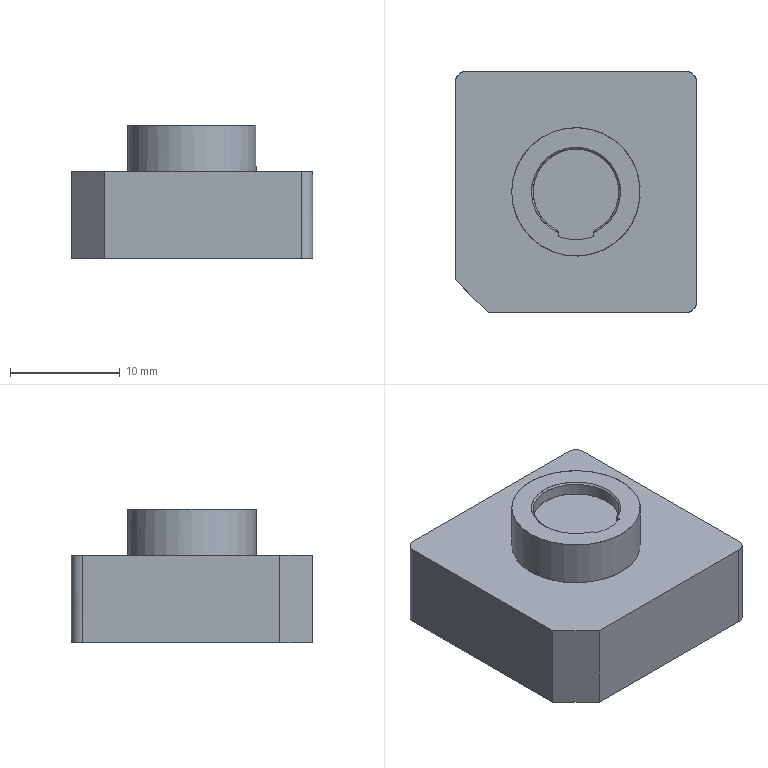NC program | PowerMill | posted by the shop | part box 22 x 22 x 12.219 mm
Lines 5490 to 7067 of 55612:
( TOOL ID   D2_1_1 )
( TOOL DIA. 2. TIP RAD 0 LENGTH 59.36 )
( Z = -4.39 )
T12 M6
T17
G91 G28 Z0
G0 G90 G54
M08
S18000 M3
X0 Y0 M8
G43 Z10.799 H12
X1.165 Y-7.017
Z.919
G1 Z-.281 F900
X1.159 Y-6.982 F1500
X1.149 Y-6.947
X1.136 Y-6.914
X1.119 Y-6.883
X1.098 Y-6.853
X1.075 Y-6.827
X1.048 Y-6.803
X1.019 Y-6.782
X.988 Y-6.764
X.955 Y-6.75
X.921 Y-6.74
X.886 Y-6.734
X.85 Y-6.731
X.815 Y-6.733
X.812
X.654 Y-6.75
X.495 Y-6.764
X.33 Y-6.774
X.171 Y-6.78
X.012 Y-6.782
X-.151 Y-6.78
X-.315 Y-6.775
X-.479 Y-6.765
X-.643 Y-6.751
X-.808 Y-6.734
X-.971 Y-6.712
X-1.133 Y-6.687
X-1.294 Y-6.657
X-1.455 Y-6.624
X-1.615 Y-6.587
X-1.775 Y-6.546
X-1.933 Y-6.501
X-2.09 Y-6.452
X-2.247 Y-6.399
X-2.401 Y-6.343
X-2.555 Y-6.282
X-2.707 Y-6.218
X-2.857 Y-6.151
X-3.006 Y-6.08
X-3.152 Y-6.005
X-3.297 Y-5.927
X-3.437 Y-5.847
X-3.575 Y-5.763
X-3.713 Y-5.675
X-3.851 Y-5.583
X-3.986 Y-5.487
X-4.117 Y-5.389
X-4.245 Y-5.289
X-4.371 Y-5.185
X-4.496 Y-5.078
X-4.617 Y-4.968
X-4.735 Y-4.855
X-4.851 Y-4.739
X-4.965 Y-4.62
X-5.076 Y-4.498
X-5.184 Y-4.373
X-5.289 Y-4.245
X-5.389 Y-4.118
X-5.485 Y-3.989
X-5.579 Y-3.856
X-5.671 Y-3.719
X-5.76 Y-3.58
X-5.846 Y-3.438
X-5.928 Y-3.295
X-6.005 Y-3.152
X-6.078 Y-3.009
X-6.148 Y-2.864
X-6.215 Y-2.714
X-6.279 Y-2.562
X-6.34 Y-2.409
X-6.397 Y-2.253
X-6.45 Y-2.097
X-6.499 Y-1.94
X-6.543 Y-1.784
X-6.584 Y-1.628
X-6.621 Y-1.471
X-6.654 Y-1.31
X-6.684 Y-1.15
X-6.709 Y-.992
X-6.731 Y-.833
X-6.749 Y-.674
X-6.763 Y-.513
X-6.773 Y-.351
X-6.779 Y-.191
X-6.782 Y-.03
X-6.781 Y.13
X-6.776 Y.293
X-6.767 Y.457
X-6.754 Y.62
X-6.737 Y.783
X-6.716 Y.946
X-6.691 Y1.109
X-6.662 Y1.272
X-6.629 Y1.433
X-6.592 Y1.594
X-6.552 Y1.753
X-6.507 Y1.911
X-6.459 Y2.068
X-6.407 Y2.224
X-6.351 Y2.379
X-6.291 Y2.533
X-6.23 Y2.681
X-6.164 Y2.828
X-6.094 Y2.977
X-6.02 Y3.123
X-5.945 Y3.264
X-5.866 Y3.404
X-5.782 Y3.545
X-5.694 Y3.684
X-5.603 Y3.821
X-5.509 Y3.955
X-5.412 Y4.088
X-5.311 Y4.218
X-5.207 Y4.346
X-5.101 Y4.47
X-4.991 Y4.592
X-4.879 Y4.711
X-4.763 Y4.828
X-4.644 Y4.942
X-4.524 Y5.053
X-4.401 Y5.16
X-4.275 Y5.265
X-4.146 Y5.367
X-4.014 Y5.467
X-3.879 Y5.563
X-3.743 Y5.656
X-3.604 Y5.745
X-3.464 Y5.831
X-3.322 Y5.913
X-3.178 Y5.992
X-3.033 Y6.066
X-2.884 Y6.138
X-2.734 Y6.206
X-2.583 Y6.271
X-2.43 Y6.332
X-2.276 Y6.389
X-2.12 Y6.442
X-1.963 Y6.492
X-1.804 Y6.538
X-1.644 Y6.58
X-1.489 Y6.617
X-1.333 Y6.65
X-1.174 Y6.68
X-1.011 Y6.706
X-.846 Y6.729
X-.683 Y6.748
X-.522 Y6.762
X-.363 Y6.773
X-.203 Y6.779
X-.042 Y6.782
X.123 Y6.781
X.288 Y6.776
X.45 Y6.767
X.611 Y6.755
X.771 Y6.738
X.934 Y6.717
X1.097 Y6.693
X1.259 Y6.664
X1.42 Y6.632
X1.581 Y6.595
X1.74 Y6.555
X1.897 Y6.511
X2.051 Y6.464
X2.202 Y6.414
X2.352 Y6.361
X2.5 Y6.304
X2.648 Y6.244
X2.793 Y6.18
X2.937 Y6.113
X3.08 Y6.042
X3.224 Y5.967
X3.366 Y5.888
X3.504 Y5.807
X3.64 Y5.723
X3.774 Y5.635
X3.91 Y5.542
X4.04 Y5.447
X4.168 Y5.35
X4.296 Y5.248
X4.421 Y5.143
X4.544 Y5.035
X4.66 Y4.928
X4.773 Y4.818
X4.886 Y4.703
X4.999 Y4.582
X5.11 Y4.459
X5.214 Y4.337
X5.314 Y4.214
X5.414 Y4.085
X5.511 Y3.953
X5.605 Y3.818
X5.696 Y3.681
X5.783 Y3.542
X5.867 Y3.401
X5.948 Y3.258
X6.026 Y3.113
X6.099 Y2.966
X6.169 Y2.817
X6.236 Y2.666
X6.299 Y2.514
X6.358 Y2.361
X6.414 Y2.205
X6.465 Y2.049
X6.513 Y1.891
X6.557 Y1.733
X6.597 Y1.574
X6.633 Y1.414
X6.665 Y1.252
X6.694 Y1.089
X6.718 Y.932
X6.738 Y.773
X6.755 Y.61
X6.767 Y.451
X6.776 Y.292
X6.781 Y.132
X6.782 Y-.027
X6.779 Y-.192
X6.773 Y-.357
X6.762 Y-.516
X6.749 Y-.675
X6.731 Y-.833
X6.709 Y-.996
X6.682 Y-1.158
X6.652 Y-1.322
X6.618 Y-1.482
X6.58 Y-1.642
X6.539 Y-1.801
X6.493 Y-1.959
X6.444 Y-2.116
X6.39 Y-2.271
X6.333 Y-2.426
X6.273 Y-2.579
X6.208 Y-2.73
X6.14 Y-2.88
X6.068 Y-3.028
X5.993 Y-3.175
X5.914 Y-3.32
X5.832 Y-3.462
X5.746 Y-3.603
X5.657 Y-3.742
X5.564 Y-3.878
X5.469 Y-4.011
X5.37 Y-4.143
X5.268 Y-4.272
X5.163 Y-4.398
X5.056 Y-4.52
X4.946 Y-4.641
X4.831 Y-4.76
X4.715 Y-4.875
X4.596 Y-4.987
X4.475 Y-5.096
X4.351 Y-5.202
X4.223 Y-5.306
X4.093 Y-5.408
X3.961 Y-5.505
X3.827 Y-5.599
X3.695 Y-5.687
X3.561 Y-5.772
X3.425 Y-5.854
X3.281 Y-5.936
X3.141 Y-6.011
X3. Y-6.083
X2.857 Y-6.151
X2.712 Y-6.216
X2.566 Y-6.278
X2.418 Y-6.336
X2.27 Y-6.391
X2.12 Y-6.442
X1.966 Y-6.491
X1.809 Y-6.536
X1.65 Y-6.578
X1.489 Y-6.617
X1.33 Y-6.65
X1.172 Y-6.68
X1.012 Y-6.706
X.848 Y-6.729
X.812 Y-6.733
X.655 Y-6.75
X.497 Y-6.764
X.332 Y-6.774
X.173 Y-6.78
X.015 Y-6.782
X-.148 Y-6.781
X-.312 Y-6.775 Z-.282
X-.476 Y-6.765
X-.64 Y-6.752
X-.805 Y-6.734
X-.968 Y-6.713
X-1.129 Y-6.687
X-1.291 Y-6.658
X-1.452 Y-6.625
X-1.612 Y-6.588 Z-.283
X-1.772 Y-6.546
X-1.926 Y-6.503
X-2.078 Y-6.456
X-2.232 Y-6.404
X-2.388 Y-6.348
X-2.539 Y-6.289
X-2.686 Y-6.227
X-2.831 Y-6.163
X-2.981 Y-6.092 Z-.284
X-3.127 Y-6.018
X-3.271 Y-5.941
X-3.413 Y-5.861
X-3.552 Y-5.778
X-3.691 Y-5.689
X-3.828 Y-5.599
X-3.96 Y-5.506
X-4.089 Y-5.411
X-4.215 Y-5.313 Z-.285
X-4.338 Y-5.213
X-4.461 Y-5.108
X-4.58 Y-5.002
X-4.697 Y-4.892
X-4.81 Y-4.781
X-4.922 Y-4.666
X-5.032 Y-4.548
X-5.14 Y-4.425
X-5.246 Y-4.298 Z-.286
X-5.346 Y-4.173
X-5.444 Y-4.044
X-5.541 Y-3.911
X-5.634 Y-3.776
X-5.722 Y-3.641
X-5.807 Y-3.503
X-5.89 Y-3.362
X-5.97 Y-3.218 Z-.287
X-6.046 Y-3.072
X-6.116 Y-2.932
X-6.182 Y-2.79
X-6.244 Y-2.647
X-6.304 Y-2.502
X-6.359 Y-2.356
X-6.412 Y-2.209
X-6.463 Y-2.056
X-6.51 Y-1.9 Z-.288
X-6.555 Y-1.742
X-6.595 Y-1.584
X-6.631 Y-1.424
X-6.663 Y-1.264
X-6.692 Y-1.102
X-6.716 Y-.944
X-6.736 Y-.786
X-6.753 Y-.627
X-6.766 Y-.466 Z-.289
X-6.775 Y-.304
X-6.78 Y-.144
X-6.782 Y.016
X-6.78 Y.176
X-6.774 Y.339
X-6.763 Y.502
X-6.749 Y.666
X-6.731 Y.829
X-6.709 Y.992 Z-.29
X-6.683 Y1.155
X-6.653 Y1.316
X-6.619 Y1.477
X-6.581 Y1.637
X-6.54 Y1.797
X-6.494 Y1.955
X-6.445 Y2.113
X-6.391 Y2.269
X-6.335 Y2.423 Z-.291
X-6.274 Y2.575
X-6.21 Y2.727
X-6.142 Y2.877
X-6.07 Y3.025
X-5.995 Y3.171
X-5.917 Y3.315
X-5.835 Y3.457
X-5.753 Y3.592 Z-.292
X-5.668 Y3.724
X-5.58 Y3.855
X-5.489 Y3.984
X-5.395 Y4.11
X-5.298 Y4.234
X-5.198 Y4.356
X-5.092 Y4.479
X-4.983 Y4.601
X-4.87 Y4.72 Z-.293
X-4.755 Y4.836
X-4.636 Y4.951
X-4.514 Y5.062
X-4.39 Y5.17
X-4.265 Y5.273
X-4.137 Y5.374
X-4.006 Y5.473
X-3.871 Y5.569
X-3.736 Y5.66 Z-.294
X-3.599 Y5.748
X-3.461 Y5.833
X-3.318 Y5.915
X-3.174 Y5.994
X-3.027 Y6.069
X-2.878 Y6.141
X-2.728 Y6.209
X-2.577 Y6.274 Z-.295
X-2.424 Y6.334
X-2.274 Y6.39
X-2.122 Y6.442
X-1.967 Y6.491
X-1.81 Y6.536
X-1.655 Y6.577
X-1.5 Y6.614
X-1.342 Y6.648
X-1.184 Y6.678 Z-.296
X-1.023 Y6.704
X-.864 Y6.727
X-.707 Y6.745
X-.551 Y6.76
X-.39 Y6.771
X-.227 Y6.778
X-.069 Y6.782
X.088
X.249 Y6.778 Z-.297
X.411 Y6.77
X.576 Y6.757
X.741 Y6.741
X.905 Y6.721
X1.065 Y6.698
X1.224 Y6.671
X1.381 Y6.64
X1.539 Y6.605
X1.698 Y6.566 Z-.298
X1.853 Y6.524
X2.006 Y6.479
X2.158 Y6.429
X2.31 Y6.376
X2.462 Y6.319
X2.611 Y6.259
X2.758 Y6.196
X2.904 Y6.129
X3.052 Y6.057 Z-.299
X3.198 Y5.981
X3.342 Y5.901
X3.484 Y5.818
X3.625 Y5.732
X3.763 Y5.642
X3.899 Y5.549
X4.032 Y5.453
X4.161 Y5.356 Z-.3
X4.287 Y5.255
X4.412 Y5.151
X4.533 Y5.044
X4.652 Y4.935
X4.767 Y4.824
X4.88 Y4.71
X4.99 Y4.593
X5.097 Y4.474
X5.201 Y4.352 Z-.301
X5.304 Y4.227
X5.404 Y4.098
X5.501 Y3.966
X5.596 Y3.831
X5.688 Y3.693
X5.776 Y3.554
X5.861 Y3.412
X5.942 Y3.27
X6.018 Y3.127 Z-.302
X6.091 Y2.982
X6.161 Y2.834
X6.228 Y2.684
X6.292 Y2.531
X6.352 Y2.377
X6.408 Y2.222
X6.458 Y2.071
X6.505 Y1.918
X6.549 Y1.761 Z-.303
X6.59 Y1.601
X6.627 Y1.44
X6.66 Y1.281
X6.688 Y1.123
X6.713 Y.965
X6.734 Y.806
X6.751 Y.645
X6.765 Y.482 Z-.304
X6.774 Y.322
X6.78 Y.161
X6.782 Y0
X6.78 Y-.164
X6.774 Y-.329
X6.764 Y-.493
X6.75 Y-.658
X6.732 Y-.821
X6.71 Y-.984 Z-.305
X6.684 Y-1.147
X6.655 Y-1.309
X6.621 Y-1.468
X6.584 Y-1.628
X6.543 Y-1.786
X6.498 Y-1.943
X6.449 Y-2.099
X6.396 Y-2.256
X6.339 Y-2.411 Z-.306
X6.279 Y-2.563
X6.216 Y-2.713
X6.149 Y-2.86
X6.079 Y-3.007
X6.004 Y-3.154
X5.928 Y-3.296
X5.847 Y-3.436
X5.762 Y-3.577 Z-.307
X5.673 Y-3.716
X5.581 Y-3.853
X5.486 Y-3.987
X5.388 Y-4.119
X5.286 Y-4.249
X5.182 Y-4.375
X5.074 Y-4.5
X4.964 Y-4.622
X4.85 Y-4.741 Z-.308
X4.733 Y-4.857
X4.623 Y-4.962
X4.511 Y-5.064
X4.397 Y-5.164
X4.28 Y-5.261
X4.161 Y-5.356
X4.032 Y-5.454
X3.9 Y-5.549
X3.765 Y-5.641 Z-.309
X3.627 Y-5.731
X3.491 Y-5.815
X3.352 Y-5.896
X3.21 Y-5.974
X3.063 Y-6.051
X2.92 Y-6.121
X2.774 Y-6.189
X2.625 Y-6.253
X2.473 Y-6.315 Z-.31
X2.318 Y-6.373
X2.162 Y-6.428
X2.005 Y-6.479
X1.848 Y-6.525
X1.692 Y-6.568
X1.54 Y-6.605
X1.388 Y-6.639
X1.227 Y-6.67
X1.067 Y-6.698 Z-.311
X.912 Y-6.721
X.812 Y-6.733
X.651 Y-6.751
X.489 Y-6.764
X.325 Y-6.774
X.16 Y-6.78
X-.005 Y-6.782
X-.17 Y-6.78
X-.333 Y-6.774 Z-.312
X-.495 Y-6.764
X-.66 Y-6.75
X-.824 Y-6.732
X-.987 Y-6.71
X-1.149 Y-6.684
X-1.311 Y-6.654
X-1.472 Y-6.62
X-1.632 Y-6.583 Z-.313
X-1.791 Y-6.541
X-1.949 Y-6.496
X-2.107 Y-6.447
X-2.263 Y-6.393
X-2.417 Y-6.337
X-2.571 Y-6.276
X-2.722 Y-6.212
X-2.872 Y-6.144
X-3.021 Y-6.072 Z-.314
X-3.167 Y-5.997
X-3.31 Y-5.919
X-3.45 Y-5.839
X-3.587 Y-5.756
X-3.725 Y-5.668
X-3.858 Y-5.578
X-3.989 Y-5.485
X-4.117 Y-5.39
X-4.242 Y-5.292 Z-.315
X-4.365 Y-5.191
X-4.487 Y-5.085
X-4.605 Y-4.979
X-4.721 Y-4.869
X-4.834 Y-4.757
X-4.945 Y-4.641
X-5.055 Y-4.521
X-5.163 Y-4.398
X-5.269 Y-4.271 Z-.316
X-5.368 Y-4.145
X-5.466 Y-4.016
X-5.561 Y-3.882
X-5.654 Y-3.746
X-5.741 Y-3.61
X-5.826 Y-3.473
X-5.908 Y-3.331
X-5.987 Y-3.187 Z-.317
X-6.062 Y-3.04
X-6.131 Y-2.9
X-6.196 Y-2.758
X-6.258 Y-2.615
X-6.316 Y-2.47
X-6.371 Y-2.324
X-6.423 Y-2.176
X-6.474 Y-2.022
X-6.52 Y-1.866 Z-.318
X-6.564 Y-1.708
X-6.603 Y-1.549
X-6.638 Y-1.39
X-6.67 Y-1.229
X-6.698 Y-1.067
X-6.721 Y-.909
X-6.74 Y-.75
X-6.756 Y-.591
X-6.769 Y-.43 Z-.319
X-6.777 Y-.268
X-6.781 Y-.108
X-6.782 Y.051
X-6.779 Y.211
X-6.772 Y.371
X-6.761 Y.532
X-6.747 Y.692
X-6.728 Y.851
X-6.706 Y1.013 Z-.32
X-6.68 Y1.175
X-6.649 Y1.337
X-6.614 Y1.498
X-6.576 Y1.658
X-6.534 Y1.816
X-6.489 Y1.973
X-6.439 Y2.129
X-6.386 Y2.285
X-6.328 Y2.439 Z-.321
X-6.267 Y2.592
X-6.203 Y2.743
X-6.134 Y2.893
X-6.062 Y3.041
X-5.989 Y3.183
X-5.912 Y3.323
X-5.832 Y3.461
X-5.749 Y3.598 Z-.322
X-5.663 Y3.732
X-5.573 Y3.865
X-5.479 Y3.997
X-5.383 Y4.125
X-5.285 Y4.251
X-5.182 Y4.376
X-5.076 Y4.498
X-4.966 Y4.619
X-4.853 Y4.737 Z-.323
X-4.738 Y4.853
X-4.619 Y4.966
X-4.497 Y5.076
X-4.373 Y5.184
X-4.247 Y5.288
X-4.118 Y5.389
X-3.986 Y5.487
X-3.851 Y5.582
X-3.715 Y5.674 Z-.324
X-3.578 Y5.762
X-3.446 Y5.841
X-3.312 Y5.918
X-3.177 Y5.992
X-3.04 Y6.062
X-2.902 Y6.13
X-2.754 Y6.198
X-2.604 Y6.262
X-2.452 Y6.323 Z-.325
X-2.302 Y6.38
X-2.151 Y6.432
X-1.997 Y6.481
X-1.84 Y6.528
X-1.685 Y6.569
X-1.529 Y6.607
X-1.372 Y6.642
X-1.214 Y6.672
X-1.053 Y6.7 Z-.326
X-.894 Y6.723
X-.738 Y6.742
X-.581 Y6.757
X-.422 Y6.769
X-.258 Y6.777
X-.1 Y6.781
X.057 Y6.782
X.22 Y6.779 Z-.327
X.384 Y6.771
X.548 Y6.76
X.713 Y6.744
X.877 Y6.725
X1.04 Y6.702
X1.202 Y6.675
X1.361 Y6.644
X1.522 Y6.609
X1.682 Y6.57 Z-.328
X1.841 Y6.528
X1.997 Y6.481
X2.15 Y6.432
X2.301 Y6.38
X2.45 Y6.324
X2.601 Y6.264
X2.748 Y6.201
X2.893 Y6.134
X3.037 Y6.064 Z-.329
X3.181 Y5.99
X3.325 Y5.911
X3.467 Y5.829
X3.608 Y5.742
X3.747 Y5.653
X3.882 Y5.561
X4.013 Y5.467
X4.142 Y5.37
X4.269 Y5.27 Z-.33
X4.394 Y5.167
X4.515 Y5.06
X4.634 Y4.952
X4.75 Y4.841
X4.863 Y4.728
X4.973 Y4.612
X5.08 Y4.493
X5.185 Y4.372 Z-.331
X5.287 Y4.248
X5.387 Y4.12
X5.485 Y3.989
X5.581 Y3.854
X5.673 Y3.717
X5.762 Y3.577
X5.847 Y3.436
X5.929 Y3.294
X6.006 Y3.151 Z-.332
X6.079 Y3.006
X6.15 Y2.859
X6.218 Y2.709
X6.282 Y2.556
X6.342 Y2.403
X6.399 Y2.248
X6.451 Y2.093
X6.499 Y1.94
X6.543 Y1.784 Z-.333
X6.585 Y1.625
X6.622 Y1.464
X6.656 Y1.304
X6.685 Y1.146
X6.71 Y.988
X6.731 Y.828
X6.749 Y.668
X6.763 Y.506
X6.773 Y.345 Z-.334
X6.779 Y.184
X6.782 Y.023
X6.78 Y-.142
X6.775 Y-.307
X6.766 Y-.473
X6.752 Y-.637
X6.736 Y-.791
X6.716 Y-.945 Z-.335
X6.692 Y-1.099
X6.663 Y-1.263
X6.632 Y-1.418
X6.598 Y-1.569
X6.561 Y-1.719
X6.517 Y-1.877
X6.47 Y-2.035
X6.418 Y-2.192
X6.363 Y-2.347 Z-.336
X6.304 Y-2.5
X6.243 Y-2.65
X6.177 Y-2.799
X6.107 Y-2.949
X6.034 Y-3.096
X5.958 Y-3.241
X5.878 Y-3.384
X5.794 Y-3.524
X5.707 Y-3.664 Z-.337
X5.616 Y-3.802
X5.522 Y-3.937
X5.425 Y-4.07
X5.325 Y-4.201
X5.221 Y-4.328
X5.115 Y-4.454
X5.005 Y-4.576
X4.893 Y-4.696 Z-.338
X4.777 Y-4.814
X4.659 Y-4.928
X4.548 Y-5.031
X4.434 Y-5.132
X4.318 Y-5.23
X4.2 Y-5.325
X4.071 Y-5.424
X3.94 Y-5.52
X3.806 Y-5.613 Z-.339
X3.669 Y-5.704
X3.528 Y-5.792
X3.391 Y-5.874
X3.25 Y-5.953
X3.104 Y-6.03
X2.961 Y-6.101
X2.816 Y-6.17
X2.668 Y-6.235
X2.516 Y-6.298 Z-.34
X2.362 Y-6.357
X2.206 Y-6.413
X2.05 Y-6.465
X1.893 Y-6.513
X1.737 Y-6.556
X1.585 Y-6.594
X1.432 Y-6.629
X1.274 Y-6.661
X1.112 Y-6.69 Z-.341
X.957 Y-6.714
X.812 Y-6.733
X.655 Y-6.75
X.497 Y-6.764
X.332 Y-6.774
X.173 Y-6.78
X.015 Y-6.782
X-.148 Y-6.781
X-.312 Y-6.775 Z-.342
X-.476 Y-6.765
X-.64 Y-6.752
X-.805 Y-6.734
X-.968 Y-6.713
X-1.129 Y-6.687
X-1.291 Y-6.658
X-1.452 Y-6.625
X-1.612 Y-6.588
X-1.772 Y-6.546 Z-.343
X-1.926 Y-6.503
X-2.078 Y-6.456
X-2.232 Y-6.404
X-2.388 Y-6.348
X-2.539 Y-6.289
X-2.686 Y-6.227
X-2.832 Y-6.162
X-2.981 Y-6.092 Z-.344
X-3.128 Y-6.018
X-3.272 Y-5.941
X-3.413 Y-5.861
X-3.552 Y-5.777
X-3.692 Y-5.689
X-3.828 Y-5.598
X-3.961 Y-5.505
X-4.089 Y-5.411
X-4.215 Y-5.313 Z-.345
X-4.339 Y-5.212
X-4.462 Y-5.108
X-4.581 Y-5.001
X-4.697 Y-4.892
X-4.811 Y-4.78
X-4.922 Y-4.666
X-5.032 Y-4.547
X-5.14 Y-4.424
X-5.246 Y-4.298 Z-.346
X-5.349 Y-4.17
X-5.448 Y-4.039
X-5.544 Y-3.907
X-5.636 Y-3.772
X-5.726 Y-3.635
X-5.812 Y-3.496
X-5.894 Y-3.355
X-5.974 Y-3.211
X-6.05 Y-3.065 Z-.347
X-6.119 Y-2.925
X-6.185 Y-2.784
X-6.247 Y-2.64
X-6.306 Y-2.496
X-6.362 Y-2.35
X-6.414 Y-2.203
X-6.465 Y-2.049
X-6.512 Y-1.894 Z-.348
X-6.556 Y-1.735
X-6.596 Y-1.577
X-6.632 Y-1.418
X-6.664 Y-1.258
X-6.693 Y-1.096
X-6.717 Y-.933
X-6.738 Y-.771
X-6.755 Y-.608
X-6.767 Y-.445 Z-.349
X-6.776 Y-.282
X-6.781 Y-.118
X-6.782 Y.046
X-6.779 Y.211
X-6.772 Y.374
X-6.761 Y.538
X-6.746 Y.701
X-6.727 Y.864
X-6.704 Y1.027 Z-.35
X-6.677 Y1.19
X-6.646 Y1.352
X-6.611 Y1.513
X-6.573 Y1.673
X-6.53 Y1.831
X-6.484 Y1.989
X-6.434 Y2.146
X-6.38 Y2.301 Z-.351
X-6.322 Y2.455
X-6.261 Y2.608
X-6.197 Y2.757
X-6.129 Y2.904
X-6.057 Y3.05
X-5.982 Y3.195
X-5.904 Y3.337
X-5.823 Y3.476
X-5.741 Y3.61 Z-.352
X-5.656 Y3.742
X-5.568 Y3.872
X-5.477 Y4.
X-5.383 Y4.126
X-5.286 Y4.249
X-5.183 Y4.374
X-5.078 Y4.496
X-4.968 Y4.617
X-4.855 Y4.735 Z-.353
X-4.74 Y4.851
X-4.621 Y4.964
X-4.499 Y5.075
X-4.375 Y5.183
X-4.249 Y5.286
X-4.12 Y5.387
X-3.988 Y5.486
X-3.853 Y5.581
X-3.717 Y5.673 Z-.354
X-3.579 Y5.761
X-3.448 Y5.84
X-3.314 Y5.917
X-3.179 Y5.991
X-3.042 Y6.061
X-2.904 Y6.129
X-2.756 Y6.197
X-2.606 Y6.261
X-2.454 Y6.323 Z-.355
X-2.304 Y6.379
X-2.153 Y6.431
X-1.999 Y6.481
X-1.842 Y6.527
X-1.687 Y6.569
X-1.532 Y6.607
X-1.374 Y6.641
X-1.217 Y6.672
X-1.056 Y6.699 Z-.356
X-.896 Y6.722
X-.74 Y6.742
X-.583 Y6.757
X-.425 Y6.769
X-.26 Y6.777
X-.103 Y6.781
X.054 Y6.782
X.21 Y6.779
X.366 Y6.772 Z-.357
X.521 Y6.762
X.677 Y6.748
X.832 Y6.731
X.995 Y6.709
X1.157 Y6.683
X1.318 Y6.653
X1.472 Y6.62
X1.626 Y6.584 Z-.358
X1.779 Y6.545
X1.932 Y6.501
X2.083 Y6.454
X2.233 Y6.404
X2.381 Y6.35
X2.534 Y6.291
X2.685 Y6.228
X2.835 Y6.161
X2.983 Y6.091 Z-.359
X3.13 Y6.016
X3.276 Y5.938
X3.42 Y5.857
X3.56 Y5.773
X3.698 Y5.685
X3.834 Y5.594
X3.969 Y5.499
X4.101 Y5.402
X4.23 Y5.301 Z-.36
X4.357 Y5.197
X4.483 Y5.089
X4.605 Y4.979
X4.719 Y4.871
X4.83 Y4.761
X4.945 Y4.642
X5.051 Y4.525
X5.155 Y4.407
X5.255 Y4.287 Z-.361
X5.357 Y4.159
X5.456 Y4.028
X5.552 Y3.895
X5.645 Y3.759
X5.735 Y3.621
X5.821 Y3.48
X5.903 Y3.339
X5.982 Y3.195 Z-.362
X6.057 Y3.05
X6.13 Y2.902
X6.199 Y2.752
X6.264 Y2.6
X6.325 Y2.446
X6.383 Y2.293
X6.436 Y2.139
X6.484 Y1.987
X6.53 Y1.832 Z-.363
X6.572 Y1.673
X6.611 Y1.512
X6.646 Y1.352
X6.676 Y1.194
X6.702 Y1.036
X6.725 Y.878
X6.744 Y.718
X6.759 Y.555
X6.771 Y.394 Z-.364
X6.778 Y.234
X6.782 Y.073
X6.781 Y-.091
X6.777 Y-.256
X6.769 Y-.42
X6.757 Y-.585
X6.741 Y-.748
X6.721 Y-.912
X6.696 Y-1.074 Z-.365
X6.668 Y-1.237
X6.637 Y-1.396
X6.601 Y-1.556
X6.562 Y-1.714
X6.519 Y-1.871
X6.472 Y-2.028
X6.421 Y-2.184
X6.366 Y-2.34 Z-.366
X6.307 Y-2.494
X6.245 Y-2.645
X6.18 Y-2.793
X6.112 Y-2.939
X6.039 Y-3.087
X5.963 Y-3.231
X5.884 Y-3.372
X5.802 Y-3.511
X5.715 Y-3.651 Z-.367
X5.625 Y-3.789
X5.531 Y-3.925
X5.434 Y-4.058
X5.334 Y-4.188
X5.231 Y-4.316
X5.125 Y-4.442
X5.017 Y-4.564
X4.905 Y-4.684
X4.789 Y-4.802 Z-.368
X4.67 Y-4.918
X4.549 Y-5.03
X4.426 Y-5.138
X4.303 Y-5.242
X4.177 Y-5.343
X4.048 Y-5.442
X3.914 Y-5.539
X3.778 Y-5.632 Z-.369
X3.641 Y-5.722
X3.504 Y-5.806
X3.365 Y-5.888
X3.222 Y-5.968
X3.075 Y-6.045
X2.929 Y-6.117
X2.78 Y-6.186
X2.63 Y-6.252
X2.477 Y-6.313 Z-.37
X2.323 Y-6.372
X2.166 Y-6.427
X2.013 Y-6.477
X1.856 Y-6.523
X1.698 Y-6.566
X1.543 Y-6.604
X1.388 Y-6.638
X1.228 Y-6.67
X1.067 Y-6.698 Z-.371
X.909 Y-6.721
X.812 Y-6.733
X.655 Y-6.75
X.497 Y-6.764
X.332 Y-6.774
X.173 Y-6.78
X.015 Y-6.782
X-.148 Y-6.781
X-.312 Y-6.775 Z-.372
X-.476 Y-6.765
X-.64 Y-6.752
X-.805 Y-6.734
X-.968 Y-6.713
X-1.13 Y-6.687
X-1.292 Y-6.658
X-1.452 Y-6.625
X-1.612 Y-6.588
X-1.771 Y-6.547 Z-.373
X-1.928 Y-6.502
X-2.083 Y-6.454
X-2.237 Y-6.402
X-2.391 Y-6.347
X-2.543 Y-6.287
X-2.693 Y-6.224
X-2.841 Y-6.158
X-2.983 Y-6.091 Z-.374
X-3.124 Y-6.02
X-3.262 Y-5.946
X-3.399 Y-5.869
X-3.534 Y-5.788
X-3.673 Y-5.702
X-3.809 Y-5.611
X-3.944 Y-5.518
X-4.072 Y-5.423
X-4.198 Y-5.326 Z-.375
X-4.322 Y-5.226
X-4.445 Y-5.123
X-4.565 Y-5.016
X-4.681 Y-4.907
X-4.795 Y-4.796
X-4.906 Y-4.682
X-5.016 Y-4.564
X-5.125 Y-4.442
X-5.231 Y-4.317 Z-.376
X-5.334 Y-4.189
X-5.434 Y-4.058
X-5.53 Y-3.926
X-5.623 Y-3.791
X-5.713 Y-3.655
X-5.8 Y-3.516
X-5.883 Y-3.375
X-5.963 Y-3.232
X-6.039 Y-3.086 Z-.377
X-6.109 Y-2.946
X-6.175 Y-2.805
X-6.238 Y-2.662
X-6.298 Y-2.517
X-6.354 Y-2.371
X-6.407 Y-2.224
X-6.458 Y-2.071
X-6.506 Y-1.916
X-6.55 Y-1.758 Z-.378
X-6.591 Y-1.598
X-6.628 Y-1.438
X-6.661 Y-1.278
X-6.689 Y-1.117
X-6.714 Y-.959
X-6.735 Y-.8
X-6.752 Y-.64
X-6.765 Y-.479 Z-.379
X-6.775 Y-.318
X-6.78 Y-.157
X-6.782 Y.003
X-6.78 Y.163
X-6.774 Y.326
X-6.764 Y.49
X-6.751 Y.653
X-6.733 Y.817
X-6.711 Y.98 Z-.38
X-6.685 Y1.142
X-6.655 Y1.304
X-6.622 Y1.466
X-6.584 Y1.627
X-6.543 Y1.786
X-6.498 Y1.944
X-6.449 Y2.101
X-6.396 Y2.257
X-6.339 Y2.411 Z-.381
X-6.279 Y2.564
X-6.215 Y2.716
X-6.147 Y2.866
X-6.075 Y3.015
X-6.001 Y3.161
X-5.922 Y3.305
X-5.841 Y3.447
X-5.756 Y3.587 Z-.382
X-5.667 Y3.726
X-5.575 Y3.863
X-5.479 Y3.997
X-5.38 Y4.129
X-5.278 Y4.258
X-5.173 Y4.385
X-5.065 Y4.51
X-4.954 Y4.631
X-4.841 Y4.75 Z-.383
X-4.724 Y4.866
X-4.604 Y4.98
X-4.482 Y5.09
X-4.357 Y5.197
X-4.231 Y5.301
X-4.101 Y5.401
X-3.969 Y5.499
X-3.834 Y5.594
X-3.698 Y5.685 Z-.384
X-3.56 Y5.773
X-3.428 Y5.852
X-3.294 Y5.928
X-3.159 Y6.002
X-3.022 Y6.072
X-2.883 Y6.139
X-2.735 Y6.206
X-2.585 Y6.27
X-2.432 Y6.331 Z-.385
X-2.282 Y6.387
X-2.13 Y6.439
X-1.976 Y6.488
X-1.819 Y6.534
X-1.664 Y6.575
X-1.509 Y6.612
X-1.351 Y6.646
X-1.193 Y6.676 Z-.386
X-1.032 Y6.703
X-.873 Y6.726
X-.717 Y6.744
X-.56 Y6.759
X-.4 Y6.77
X-.236 Y6.778
X-.078 Y6.782
X.079
X.242 Y6.778 Z-.387
X.406 Y6.77
X.57 Y6.758
X.735 Y6.742
X.899 Y6.722
X1.062 Y6.698
X1.223 Y6.671
X1.383 Y6.64
X1.544 Y6.604
X1.704 Y6.565 Z-.388
X1.862 Y6.521
X2.019 Y6.475
X2.173 Y6.424
X2.326 Y6.371
X2.478 Y6.313
X2.629 Y6.252
X2.778 Y6.187
X2.925 Y6.119
X3.07 Y6.048 Z-.389
X3.213 Y5.973
X3.357 Y5.893
X3.499 Y5.81
X3.639 Y5.723
X3.777 Y5.633
X3.911 Y5.541
X4.042 Y5.446
X4.171 Y5.348 Z-.39
X4.297 Y5.247
X4.422 Y5.142
X4.543 Y5.035
X4.662 Y4.926
X4.777 Y4.814
X4.889 Y4.7
X5. Y4.583
X5.106 Y4.463
X5.21 Y4.342 Z-.391
X5.312 Y4.216
X5.412 Y4.087
X5.51 Y3.955
X5.604 Y3.819
X5.696 Y3.681
X5.784 Y3.542
X5.868 Y3.4
X5.949 Y3.258
X6.025 Y3.114 Z-.392
X6.097 Y2.97
X6.167 Y2.821
X6.234 Y2.671
X6.297 Y2.518
X6.357 Y2.364
X6.412 Y2.209
X6.463 Y2.057
X6.509 Y1.904
X6.553 Y1.747 Z-.393
X6.594 Y1.587
X6.63 Y1.426
X6.663 Y1.266
X6.691 Y1.109
X6.715 Y.95
X6.736 Y.785
X6.754 Y.621
X6.767 Y.458 Z-.394
X6.776 Y.295
X6.781 Y.136
X6.782 Y-.024
X6.779 Y-.189
X6.773 Y-.354
X6.763 Y-.513
X6.749 Y-.672
X6.731 Y-.83
X6.709 Y-.992 Z-.395
X6.683 Y-1.155
X6.652 Y-1.319
X6.619 Y-1.478
X6.581 Y-1.638
X6.54 Y-1.796
X6.494 Y-1.955
X6.446 Y-2.11
X6.393 Y-2.264
X6.336 Y-2.418 Z-.396
X6.276 Y-2.571
X6.211 Y-2.724
X6.144 Y-2.872
X6.073 Y-3.019
X5.998 Y-3.166
X5.919 Y-3.31
X5.837 Y-3.454
X5.751 Y-3.595 Z-.397
X5.662 Y-3.733
X5.57 Y-3.869
X5.475 Y-4.002
X5.378 Y-4.132
X5.276 Y-4.262
X5.173 Y-4.387
X5.067 Y-4.508
X4.956 Y-4.629
X4.842 Y-4.748 Z-.398
X4.726 Y-4.865
X4.616 Y-4.969
X4.503 Y-5.071
X4.389 Y-5.171
X4.272 Y-5.268
X4.153 Y-5.362
X4.024 Y-5.46
X3.892 Y-5.554
X3.756 Y-5.647 Z-.399
X3.618 Y-5.736
X3.482 Y-5.82
X3.343 Y-5.901
X3.201 Y-5.979
X3.053 Y-6.056
X2.91 Y-6.126
X2.764 Y-6.193
X2.615 Y-6.258
X2.462 Y-6.319 Z-.4
X2.308 Y-6.377
X2.151 Y-6.432
X1.994 Y-6.482
X1.838 Y-6.528
X1.682 Y-6.57
X1.53 Y-6.607
X1.376 Y-6.641
X1.215 Y-6.672
X1.056 Y-6.699 Z-.401
X.901 Y-6.722
X.812 Y-6.733
X.651 Y-6.751
X.489 Y-6.764
X.325 Y-6.774
X.16 Y-6.78
X-.005 Y-6.782
X-.17 Y-6.78
X-.333 Y-6.774 Z-.402
X-.495 Y-6.764
X-.66 Y-6.75
X-.823 Y-6.732
X-.986 Y-6.71
X-1.149 Y-6.684
X-1.311 Y-6.654
X-1.472 Y-6.62
X-1.633 Y-6.583 Z-.403
X-1.793 Y-6.541
X-1.946 Y-6.497
X-2.098 Y-6.449
X-2.253 Y-6.397
X-2.409 Y-6.34
X-2.559 Y-6.281
X-2.706 Y-6.219
X-2.851 Y-6.153
X-3. Y-6.082 Z-.404
X-3.147 Y-6.008
X-3.29 Y-5.93
X-3.431 Y-5.85
X-3.57 Y-5.766
X-3.71 Y-5.678
X-3.846 Y-5.586
X-3.978 Y-5.493
X-4.108 Y-5.396
X-4.235 Y-5.297 Z-.405
X-4.361 Y-5.194
X-4.484 Y-5.088
X-4.605 Y-4.979
X-4.722 Y-4.868
X-4.837 Y-4.754
X-4.949 Y-4.637
X-5.059 Y-4.517
X-5.167 Y-4.393
X-5.273 Y-4.266 Z-.406
X-5.374 Y-4.137
X-5.471 Y-4.007
X-5.567 Y-3.873
X-5.66 Y-3.737
X-5.749 Y-3.598
X-5.834 Y-3.458
X-5.916 Y-3.316
X-5.995 Y-3.172 Z-.407
X-6.07 Y-3.026
X-6.138 Y-2.885
X-6.203 Y-2.743
X-6.264 Y-2.599
X-6.322 Y-2.454
X-6.377 Y-2.308
X-6.429 Y-2.161
X-6.478 Y-2.007
X-6.525 Y-1.85 Z-.408
X-6.568 Y-1.691
X-6.607 Y-1.533
X-6.642 Y-1.373
X-6.673 Y-1.212
X-6.7 Y-1.05
X-6.724 Y-.888
X-6.743 Y-.725
X-6.759 Y-.563
X-6.77 Y-.399 Z-.409
X-6.778 Y-.236
X-6.782 Y-.072
X-6.781 Y.093
X-6.777 Y.257
X-6.769 Y.421
X-6.757 Y.584
X-6.741 Y.748
X-6.721 Y.911
X-6.697 Y1.074 Z-.41
X-6.669 Y1.236
X-6.637 Y1.398
X-6.601 Y1.558
X-6.561 Y1.718
X-6.517 Y1.876
X-6.47 Y2.034
X-6.418 Y2.191
X-6.363 Y2.346 Z-.411
X-6.304 Y2.5
X-6.244 Y2.649
X-6.179 Y2.795
X-6.11 Y2.944
X-6.037 Y3.091
X-5.962 Y3.233
X-5.884 Y3.373
X-5.802 Y3.512
X-5.716 Y3.65 Z-.412
X-5.627 Y3.786
X-5.534 Y3.921
X-5.438 Y4.052
X-5.34 Y4.181
X-5.239 Y4.307
X-5.133 Y4.432
X-5.025 Y4.555
X-4.914 Y4.675
X-4.799 Y4.792 Z-.413
X-4.681 Y4.908
X-4.56 Y5.02
X-4.437 Y5.129
X-4.313 Y5.234
X-4.185 Y5.337
X-4.055 Y5.436
X-3.921 Y5.533
X-3.786 Y5.627 Z-.414
X-3.649 Y5.717
X-3.511 Y5.803
X-3.378 Y5.881
X-3.244 Y5.956
X-3.108 Y6.028
X-2.97 Y6.097
X-2.831 Y6.163
X-2.682 Y6.229
X-2.531 Y6.292 Z-.415
X-2.377 Y6.352
X-2.226 Y6.406
X-2.075 Y6.457
X-1.917 Y6.505
X-1.763 Y6.549
X-1.608 Y6.589
X-1.452 Y6.625
X-1.294 Y6.657
X-1.135 Y6.686 Z-.416
X-.975 Y6.712
X-.815 Y6.733
X-.658 Y6.75
X-.501 Y6.763
X-.339 Y6.774
X-.177 Y6.78
X-.02 Y6.782
X.136 Y6.781
X.292 Y6.776 Z-.417
X.453 Y6.767
X.609 Y6.755
X.764 Y6.739
X.927 Y6.719
X1.089 Y6.694
X1.251 Y6.666
X1.413 Y6.633
X1.566 Y6.599
X1.719 Y6.561 Z-.418
X1.87 Y6.519
X2.021 Y6.474
X2.171 Y6.425
X2.319 Y6.373
X2.471 Y6.316
X2.622 Y6.255
X2.773 Y6.189
X2.922 Y6.12
X3.069 Y6.048 Z-.419
X3.215 Y5.972
X3.359 Y5.892
X3.502 Y5.808
X3.642 Y5.721
X3.779 Y5.632
X3.914 Y5.539
X4.046 Y5.443
X4.175 Y5.345 Z-.42
X4.3 Y5.245
X4.425 Y5.14
X4.545 Y5.034
X4.663 Y4.924
X4.778 Y4.813
X4.891 Y4.699
X5.001 Y4.581
X5.107 Y4.462
X5.211 Y4.34 Z-.421
X5.313 Y4.215
X5.413 Y4.086
X5.511 Y3.953
X5.605 Y3.818
X5.697 Y3.68
X5.785 Y3.54
X5.869 Y3.399
X5.949 Y3.256
X6.026 Y3.113 Z-.422
X6.098 Y2.968
X6.168 Y2.82
X6.235 Y2.669
X6.298 Y2.516
X6.357 Y2.362
X6.413 Y2.207
X6.463 Y2.056
X6.51 Y1.902
X6.554 Y1.745 Z-.423
X6.594 Y1.585
X6.631 Y1.424
X6.663 Y1.265
X6.691 Y1.107
X6.715 Y.949
X6.736 Y.789
X6.753 Y.628
X6.766 Y.466 Z-.424
X6.775 Y.306
X6.78 Y.145
X6.782 Y-.016
X6.78 Y-.182
X6.773 Y-.347
X6.763 Y-.512
X6.748 Y-.676
X6.731 Y-.832
X6.71 Y-.988 Z-.425
X6.684 Y-1.147
X6.654 Y-1.311
X6.621 Y-1.469
X6.585 Y-1.622
X6.546 Y-1.775
X6.501 Y-1.933
X6.452 Y-2.091
X6.399 Y-2.247
X6.342 Y-2.402 Z-.426
X6.282 Y-2.556
X6.218 Y-2.708
X6.15 Y-2.858
X6.079 Y-3.007
X6.005 Y-3.153
X5.927 Y-3.297
X5.845 Y-3.44
X5.76 Y-3.581
X5.671 Y-3.72 Z-.427
X5.579 Y-3.856
X5.484 Y-3.99
X5.387 Y-4.12
X5.285 Y-4.251
X5.181 Y-4.377
X5.074 Y-4.5
X4.963 Y-4.622
X4.85 Y-4.741 Z-.428
X4.733 Y-4.858